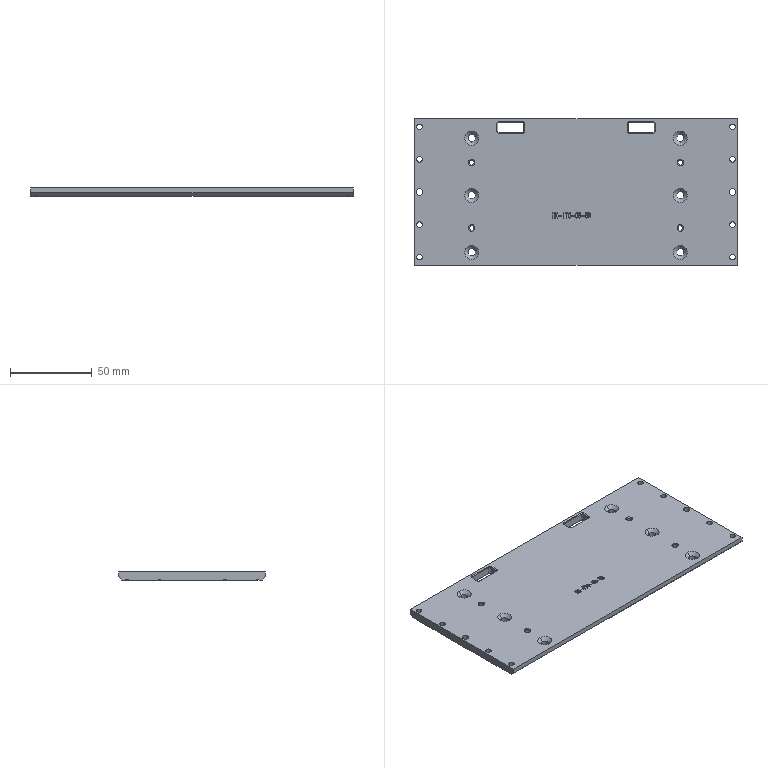NC program | NX | posted with a generic post | part box 198 x 90 x 5 mm
Lines 1352 to 3241 of 7160, first 1568 of 1886 lines:
(ZLEVEL_PROFILE_COPY_1_COPY_COPY_COPY , TOOL : D2)
N2654 T17 M6
N2656 G54
N2658 G17 G0 G90 X-34.395 Y37.9 S9500 M3
N2660 G43 Z30. H17
N2662 Z-0.2
N2664 G94 G1 X-34.222 Y37.6 F1000.
N2666 G3 X-34.048 Y37.5 R0.2
N2668 G1 X-32.9 F1100.
N2670 Y37.653
N2672 Y38.648
N2674 G3 X-33. Y38.822 R0.2
N2676 G1 X-33.3 Y38.995
N2678 G0 X-34.395 Y37.9 Z-0.4
N2680 G1 X-34.222 Y37.6 F1000.
N2682 G3 X-34.048 Y37.5 R0.2
N2684 G1 X-32.9 F1100.
N2686 Y37.653
N2688 Y38.648
N2690 G3 X-33. Y38.822 R0.2
N2692 G1 X-33.3 Y38.995
N2694 G0 X-34.395 Y37.9 Z-0.6
N2696 G1 X-34.222 Y37.6 F1000.
N2698 G3 X-34.048 Y37.5 R0.2
N2700 G1 X-32.9 F1100.
N2702 Y37.653
N2704 Y38.648
N2706 G3 X-33. Y38.822 R0.2
N2708 G1 X-33.3 Y38.995
N2710 G0 X-34.395 Y37.9 Z-0.8
N2712 G1 X-34.222 Y37.6 F1000.
N2714 G3 X-34.048 Y37.5 R0.2
N2716 G1 X-32.9 F1100.
N2718 Y37.653
N2720 Y38.648
N2722 G3 X-33. Y38.822 R0.2
N2724 G1 X-33.3 Y38.995
N2726 G0 X-34.395 Y37.9 Z-1.
N2728 G1 X-34.222 Y37.6 F1000.
N2730 G3 X-34.048 Y37.5 R0.2
N2732 G1 X-32.9 F1100.
N2734 Y37.653
N2736 Y38.648
N2738 G3 X-33. Y38.822 R0.2
N2740 G1 X-33.3 Y38.995
N2742 G0 X-34.395 Y37.9 Z-1.2
N2744 G1 X-34.222 Y37.6 F1000.
N2746 G3 X-34.048 Y37.5 R0.2
N2748 G1 X-32.9 F1100.
N2750 Y37.653
N2752 Y38.648
N2754 G3 X-33. Y38.822 R0.2
N2756 G1 X-33.3 Y38.995
N2758 G0 X-34.395 Y37.9 Z-1.4
N2760 G1 X-34.222 Y37.6 F1000.
N2762 G3 X-34.048 Y37.5 R0.2
N2764 G1 X-32.9 F1100.
N2766 Y37.653
N2768 Y38.648
N2770 G3 X-33. Y38.822 R0.2
N2772 G1 X-33.3 Y38.995
N2774 G0 X-34.395 Y37.9 Z-1.6
N2776 G1 X-34.222 Y37.6 F1000.
N2778 G3 X-34.048 Y37.5 R0.2
N2780 G1 X-32.9 F1100.
N2782 Y37.653
N2784 Y38.648
N2786 G3 X-33. Y38.822 R0.2
N2788 G1 X-33.3 Y38.995
N2790 G0 X-34.395 Y37.9 Z-1.8
N2792 G1 X-34.222 Y37.6 F1000.
N2794 G3 X-34.048 Y37.5 R0.2
N2796 G1 X-32.9 F1100.
N2798 Y37.653
N2800 Y38.648
N2802 G3 X-33. Y38.822 R0.2
N2804 G1 X-33.3 Y38.995
N2806 G0 X-34.395 Y37.9 Z-2.
N2808 G1 X-34.222 Y37.6 F1000.
N2810 G3 X-34.048 Y37.5 R0.2
N2812 G1 X-32.9 F1100.
N2814 Y37.653
N2816 Y38.648
N2818 G3 X-33. Y38.822 R0.2
N2820 G1 X-33.3 Y38.995
N2822 G0 X-34.395 Y37.9 Z-2.2
N2824 G1 X-34.222 Y37.6 F1000.
N2826 G3 X-34.048 Y37.5 R0.2
N2828 G1 X-32.9 F1100.
N2830 Y37.653
N2832 Y38.648
N2834 G3 X-33. Y38.822 R0.2
N2836 G1 X-33.3 Y38.995
N2838 G0 X-34.395 Y37.9 Z-2.4
N2840 G1 X-34.222 Y37.6 F1000.
N2842 G3 X-34.048 Y37.5 R0.2
N2844 G1 X-32.9 F1100.
N2846 Y37.653
N2848 Y38.648
N2850 G3 X-33. Y38.822 R0.2
N2852 G1 X-33.3 Y38.995
N2854 G0 X-34.395 Y37.9 Z-2.6
N2856 G1 X-34.222 Y37.6 F1000.
N2858 G3 X-34.048 Y37.5 R0.2
N2860 G1 X-32.9 F1100.
N2862 Y37.653
N2864 Y38.648
N2866 G3 X-33. Y38.822 R0.2
N2868 G1 X-33.3 Y38.995
N2870 G0 X-34.395 Y37.9 Z-2.8
N2872 G1 X-34.222 Y37.6 F1000.
N2874 G3 X-34.048 Y37.5 R0.2
N2876 G1 X-32.9 F1100.
N2878 Y37.653
N2880 Y38.648
N2882 G3 X-33. Y38.822 R0.2
N2884 G1 X-33.3 Y38.995
N2886 G0 X-34.395 Y37.9 Z-3.
N2888 G1 X-34.222 Y37.6 F1000.
N2890 G3 X-34.048 Y37.5 R0.2
N2892 G1 X-32.9 F1100.
N2894 Y37.653
N2896 Y38.648
N2898 G3 X-33. Y38.822 R0.2
N2900 G1 X-33.3 Y38.995
N2902 G0 X-34.395 Y37.9 Z-3.2
N2904 G1 X-34.222 Y37.6 F1000.
N2906 G3 X-34.048 Y37.5 R0.2
N2908 G1 X-32.9 F1100.
N2910 Y37.653
N2912 Y38.648
N2914 G3 X-33. Y38.822 R0.2
N2916 G1 X-33.3 Y38.995
N2918 G0 X-34.395 Y37.9 Z-3.4
N2920 G1 X-34.222 Y37.6 F1000.
N2922 G3 X-34.048 Y37.5 R0.2
N2924 G1 X-32.9 F1100.
N2926 Y37.653
N2928 Y38.648
N2930 G3 X-33. Y38.822 R0.2
N2932 G1 X-33.3 Y38.995
N2934 G0 X-34.395 Y37.9 Z-3.6
N2936 G1 X-34.222 Y37.6 F1000.
N2938 G3 X-34.048 Y37.5 R0.2
N2940 G1 X-32.9 F1100.
N2942 Y37.653
N2944 Y38.648
N2946 G3 X-33. Y38.822 R0.2
N2948 G1 X-33.3 Y38.995
N2950 G0 X-34.395 Y37.9 Z-3.8
N2952 G1 X-34.222 Y37.6 F1000.
N2954 G3 X-34.048 Y37.5 R0.2
N2956 G1 X-32.9 F1100.
N2958 Y37.653
N2960 Y38.648
N2962 G3 X-33. Y38.822 R0.2
N2964 G1 X-33.3 Y38.995
N2966 G0 X-34.395 Y37.9 Z-4.
N2968 G1 X-34.222 Y37.6 F1000.
N2970 G3 X-34.048 Y37.5 R0.2
N2972 G1 X-32.9 F1100.
N2974 Y37.653
N2976 Y38.648
N2978 G3 X-33. Y38.822 R0.2
N2980 G1 X-33.3 Y38.995
N2982 G0 X-34.395 Y37.9 Z-4.2
N2984 G1 X-34.222 Y37.6 F1000.
N2986 G3 X-34.048 Y37.5 R0.2
N2988 G1 X-32.9 F1100.
N2990 Y37.653
N2992 Y38.648
N2994 G3 X-33. Y38.822 R0.2
N2996 G1 X-33.3 Y38.995
N2998 G0 X-34.395 Y37.9 Z-4.4
N3000 G1 X-34.222 Y37.6 F1000.
N3002 G3 X-34.048 Y37.5 R0.2
N3004 G1 X-32.9 F1100.
N3006 Y37.653
N3008 Y38.648
N3010 G3 X-33. Y38.822 R0.2
N3012 G1 X-33.3 Y38.995
N3014 G0 X-34.395 Y37.9 Z-4.6
N3016 G1 X-34.222 Y37.6 F1000.
N3018 G3 X-34.048 Y37.5 R0.2
N3020 G1 X-32.9 F1100.
N3022 Y37.653
N3024 Y38.648
N3026 G3 X-33. Y38.822 R0.2
N3028 G1 X-33.3 Y38.995
N3030 G0 X-34.395 Y37.9 Z-4.8
N3032 G1 X-34.222 Y37.6 F1000.
N3034 G3 X-34.048 Y37.5 R0.2
N3036 G1 X-32.9 F1100.
N3038 Y37.653
N3040 Y38.648
N3042 G3 X-33. Y38.822 R0.2
N3044 G1 X-33.3 Y38.995
N3046 G0 X-34.395 Y37.9 Z-5.
N3048 G1 X-34.222 Y37.6 F1000.
N3050 G3 X-34.048 Y37.5 R0.2
N3052 G1 X-32.9 F1100.
N3054 Y37.653
N3056 Y38.648
N3058 G3 X-33. Y38.822 R0.2
N3060 G1 X-33.3 Y38.995
N3062 G0 Z30.
N3064 Y40.205
N3066 Z-0.2
N3068 G1 X-33. Y40.378 F1000.
N3070 G3 X-32.9 Y40.552 R0.2
N3072 G1 Y41.7 F1100.
N3074 X-33.046
N3076 X-34.048
N3078 G3 X-34.222 Y41.6 R0.2
N3080 G1 X-34.395 Y41.3
N3082 G0 X-33.3 Y40.205 Z-0.4
N3084 G1 X-33. Y40.378 F1000.
N3086 G3 X-32.9 Y40.552 R0.2
N3088 G1 Y41.7 F1100.
N3090 X-33.046
N3092 X-34.048
N3094 G3 X-34.222 Y41.6 R0.2
N3096 G1 X-34.395 Y41.3
N3098 G0 X-33.3 Y40.205 Z-0.6
N3100 G1 X-33. Y40.378 F1000.
N3102 G3 X-32.9 Y40.552 R0.2
N3104 G1 Y41.7 F1100.
N3106 X-33.046
N3108 X-34.048
N3110 G3 X-34.222 Y41.6 R0.2
N3112 G1 X-34.395 Y41.3
N3114 G0 X-33.3 Y40.205 Z-0.8
N3116 G1 X-33. Y40.378 F1000.
N3118 G3 X-32.9 Y40.552 R0.2
N3120 G1 Y41.7 F1100.
N3122 X-33.046
N3124 X-34.048
N3126 G3 X-34.222 Y41.6 R0.2
N3128 G1 X-34.395 Y41.3
N3130 G0 X-33.3 Y40.205 Z-1.
N3132 G1 X-33. Y40.378 F1000.
N3134 G3 X-32.9 Y40.552 R0.2
N3136 G1 Y41.7 F1100.
N3138 X-33.046
N3140 X-34.048
N3142 G3 X-34.222 Y41.6 R0.2
N3144 G1 X-34.395 Y41.3
N3146 G0 X-33.3 Y40.205 Z-1.2
N3148 G1 X-33. Y40.378 F1000.
N3150 G3 X-32.9 Y40.552 R0.2
N3152 G1 Y41.7 F1100.
N3154 X-33.046
N3156 X-34.048
N3158 G3 X-34.222 Y41.6 R0.2
N3160 G1 X-34.395 Y41.3
N3162 G0 X-33.3 Y40.205 Z-1.4
N3164 G1 X-33. Y40.378 F1000.
N3166 G3 X-32.9 Y40.552 R0.2
N3168 G1 Y41.7 F1100.
N3170 X-33.046
N3172 X-34.048
N3174 G3 X-34.222 Y41.6 R0.2
N3176 G1 X-34.395 Y41.3
N3178 G0 X-33.3 Y40.205 Z-1.6
N3180 G1 X-33. Y40.378 F1000.
N3182 G3 X-32.9 Y40.552 R0.2
N3184 G1 Y41.7 F1100.
N3186 X-33.046
N3188 X-34.048
N3190 G3 X-34.222 Y41.6 R0.2
N3192 G1 X-34.395 Y41.3
N3194 G0 X-33.3 Y40.205 Z-1.8
N3196 G1 X-33. Y40.378 F1000.
N3198 G3 X-32.9 Y40.552 R0.2
N3200 G1 Y41.7 F1100.
N3202 X-33.046
N3204 X-34.048
N3206 G3 X-34.222 Y41.6 R0.2
N3208 G1 X-34.395 Y41.3
N3210 G0 X-33.3 Y40.205 Z-2.
N3212 G1 X-33. Y40.378 F1000.
N3214 G3 X-32.9 Y40.552 R0.2
N3216 G1 Y41.7 F1100.
N3218 X-33.046
N3220 X-34.048
N3222 G3 X-34.222 Y41.6 R0.2
N3224 G1 X-34.395 Y41.3
N3226 G0 X-33.3 Y40.205 Z-2.2
N3228 G1 X-33. Y40.378 F1000.
N3230 G3 X-32.9 Y40.552 R0.2
N3232 G1 Y41.7 F1100.
N3234 X-33.046
N3236 X-34.048
N3238 G3 X-34.222 Y41.6 R0.2
N3240 G1 X-34.395 Y41.3
N3242 G0 X-33.3 Y40.205 Z-2.4
N3244 G1 X-33. Y40.378 F1000.
N3246 G3 X-32.9 Y40.552 R0.2
N3248 G1 Y41.7 F1100.
N3250 X-33.046
N3252 X-34.048
N3254 G3 X-34.222 Y41.6 R0.2
N3256 G1 X-34.395 Y41.3
N3258 G0 X-33.3 Y40.205 Z-2.6
N3260 G1 X-33. Y40.378 F1000.
N3262 G3 X-32.9 Y40.552 R0.2
N3264 G1 Y41.7 F1100.
N3266 X-33.046
N3268 X-34.048
N3270 G3 X-34.222 Y41.6 R0.2
N3272 G1 X-34.395 Y41.3
N3274 G0 X-33.3 Y40.205 Z-2.8
N3276 G1 X-33. Y40.378 F1000.
N3278 G3 X-32.9 Y40.552 R0.2
N3280 G1 Y41.7 F1100.
N3282 X-33.046
N3284 X-34.048
N3286 G3 X-34.222 Y41.6 R0.2
N3288 G1 X-34.395 Y41.3
N3290 G0 X-33.3 Y40.205 Z-3.
N3292 G1 X-33. Y40.378 F1000.
N3294 G3 X-32.9 Y40.552 R0.2
N3296 G1 Y41.7 F1100.
N3298 X-33.046
N3300 X-34.048
N3302 G3 X-34.222 Y41.6 R0.2
N3304 G1 X-34.395 Y41.3
N3306 G0 X-33.3 Y40.205 Z-3.2
N3308 G1 X-33. Y40.378 F1000.
N3310 G3 X-32.9 Y40.552 R0.2
N3312 G1 Y41.7 F1100.
N3314 X-33.046
N3316 X-34.048
N3318 G3 X-34.222 Y41.6 R0.2
N3320 G1 X-34.395 Y41.3
N3322 G0 X-33.3 Y40.205 Z-3.4
N3324 G1 X-33. Y40.378 F1000.
N3326 G3 X-32.9 Y40.552 R0.2
N3328 G1 Y41.7 F1100.
N3330 X-33.046
N3332 X-34.048
N3334 G3 X-34.222 Y41.6 R0.2
N3336 G1 X-34.395 Y41.3
N3338 G0 X-33.3 Y40.205 Z-3.6
N3340 G1 X-33. Y40.378 F1000.
N3342 G3 X-32.9 Y40.552 R0.2
N3344 G1 Y41.7 F1100.
N3346 X-33.046
N3348 X-34.048
N3350 G3 X-34.222 Y41.6 R0.2
N3352 G1 X-34.395 Y41.3
N3354 G0 X-33.3 Y40.205 Z-3.8
N3356 G1 X-33. Y40.378 F1000.
N3358 G3 X-32.9 Y40.552 R0.2
N3360 G1 Y41.7 F1100.
N3362 X-33.046
N3364 X-34.048
N3366 G3 X-34.222 Y41.6 R0.2
N3368 G1 X-34.395 Y41.3
N3370 G0 X-33.3 Y40.205 Z-4.
N3372 G1 X-33. Y40.378 F1000.
N3374 G3 X-32.9 Y40.552 R0.2
N3376 G1 Y41.7 F1100.
N3378 X-33.003
N3380 X-34.048
N3382 G3 X-34.222 Y41.6 R0.2
N3384 G1 X-34.395 Y41.3
N3386 G0 X-33.3 Y40.205 Z-4.2
N3388 G1 X-33. Y40.378 F1000.
N3390 G3 X-32.9 Y40.552 R0.2
N3392 G1 Y41.7 F1100.
N3394 X-33.003
N3396 X-34.048
N3398 G3 X-34.222 Y41.6 R0.2
N3400 G1 X-34.395 Y41.3
N3402 G0 X-33.3 Y40.205 Z-4.4
N3404 G1 X-33. Y40.378 F1000.
N3406 G3 X-32.9 Y40.552 R0.2
N3408 G1 Y41.7 F1100.
N3410 X-33.003
N3412 X-34.048
N3414 G3 X-34.222 Y41.6 R0.2
N3416 G1 X-34.395 Y41.3
N3418 G0 X-33.3 Y40.206 Z-4.6
N3420 G1 X-33. Y40.379 F1000.
N3422 G3 X-32.9 Y40.552 R0.2
N3424 G1 Y41.7 F1100.
N3426 X-34.048
N3428 G3 X-34.221 Y41.6 R0.2
N3430 G1 X-34.394 Y41.3
N3432 G0 X-33.3 Y40.206 Z-4.8
N3434 G1 X-33. Y40.379 F1000.
N3436 G3 X-32.9 Y40.552 R0.2
N3438 G1 Y41.7 F1100.
N3440 X-34.048
N3442 G3 X-34.221 Y41.6 R0.2
N3444 G1 X-34.394 Y41.3
N3446 G0 X-33.3 Y40.206 Z-5.
N3448 G1 X-33. Y40.379 F1000.
N3450 G3 X-32.9 Y40.552 R0.2
N3452 G1 Y41.7 F1100.
N3454 X-34.048
N3456 G3 X-34.221 Y41.6 R0.2
N3458 G1 X-34.394 Y41.3
N3460 G0 Z30.
N3462 X-45.605
N3464 Z-0.2
N3466 G1 X-45.778 Y41.6 F1000.
N3468 G3 X-45.952 Y41.7 R0.2
N3470 G1 X-46.954 F1100.
N3472 X-47.1
N3474 Y40.552
N3476 G3 X-47. Y40.378 R0.2
N3478 G1 X-46.7 Y40.205
N3480 G0 X-45.605 Y41.3 Z-0.4
N3482 G1 X-45.778 Y41.6 F1000.
N3484 G3 X-45.952 Y41.7 R0.2
N3486 G1 X-46.954 F1100.
N3488 X-47.1
N3490 Y40.552
N3492 G3 X-47. Y40.378 R0.2
N3494 G1 X-46.7 Y40.205
N3496 G0 X-45.605 Y41.3 Z-0.6
N3498 G1 X-45.778 Y41.6 F1000.
N3500 G3 X-45.952 Y41.7 R0.2
N3502 G1 X-46.954 F1100.
N3504 X-47.1
N3506 Y40.552
N3508 G3 X-47. Y40.378 R0.2
N3510 G1 X-46.7 Y40.205
N3512 G0 X-45.605 Y41.3 Z-0.8
N3514 G1 X-45.778 Y41.6 F1000.
N3516 G3 X-45.952 Y41.7 R0.2
N3518 G1 X-46.954 F1100.
N3520 X-47.1
N3522 Y40.552
N3524 G3 X-47. Y40.378 R0.2
N3526 G1 X-46.7 Y40.205
N3528 G0 X-45.605 Y41.3 Z-1.
N3530 G1 X-45.778 Y41.6 F1000.
N3532 G3 X-45.952 Y41.7 R0.2
N3534 G1 X-46.954 F1100.
N3536 X-47.1
N3538 Y40.552
N3540 G3 X-47. Y40.378 R0.2
N3542 G1 X-46.7 Y40.205
N3544 G0 X-45.605 Y41.3 Z-1.2
N3546 G1 X-45.778 Y41.6 F1000.
N3548 G3 X-45.952 Y41.7 R0.2
N3550 G1 X-46.954 F1100.
N3552 X-47.1
N3554 Y40.552
N3556 G3 X-47. Y40.378 R0.2
N3558 G1 X-46.7 Y40.205
N3560 G0 X-45.605 Y41.3 Z-1.4
N3562 G1 X-45.778 Y41.6 F1000.
N3564 G3 X-45.952 Y41.7 R0.2
N3566 G1 X-46.954 F1100.
N3568 X-47.1
N3570 Y40.552
N3572 G3 X-47. Y40.378 R0.2
N3574 G1 X-46.7 Y40.205
N3576 G0 X-45.605 Y41.3 Z-1.6
N3578 G1 X-45.778 Y41.6 F1000.
N3580 G3 X-45.952 Y41.7 R0.2
N3582 G1 X-46.954 F1100.
N3584 X-47.1
N3586 Y40.552
N3588 G3 X-47. Y40.378 R0.2
N3590 G1 X-46.7 Y40.205
N3592 G0 X-45.605 Y41.3 Z-1.8
N3594 G1 X-45.778 Y41.6 F1000.
N3596 G3 X-45.952 Y41.7 R0.2
N3598 G1 X-46.954 F1100.
N3600 X-47.1
N3602 Y40.552
N3604 G3 X-47. Y40.378 R0.2
N3606 G1 X-46.7 Y40.205
N3608 G0 X-45.605 Y41.3 Z-2.
N3610 G1 X-45.778 Y41.6 F1000.
N3612 G3 X-45.952 Y41.7 R0.2
N3614 G1 X-46.954 F1100.
N3616 X-47.1
N3618 Y40.552
N3620 G3 X-47. Y40.378 R0.2
N3622 G1 X-46.7 Y40.205
N3624 G0 X-45.605 Y41.3 Z-2.2
N3626 G1 X-45.778 Y41.6 F1000.
N3628 G3 X-45.952 Y41.7 R0.2
N3630 G1 X-46.954 F1100.
N3632 X-47.1
N3634 Y40.552
N3636 G3 X-47. Y40.378 R0.2
N3638 G1 X-46.7 Y40.205
N3640 G0 X-45.605 Y41.3 Z-2.4
N3642 G1 X-45.778 Y41.6 F1000.
N3644 G3 X-45.952 Y41.7 R0.2
N3646 G1 X-46.954 F1100.
N3648 X-47.1
N3650 Y40.552
N3652 G3 X-47. Y40.378 R0.2
N3654 G1 X-46.7 Y40.205
N3656 G0 X-45.605 Y41.3 Z-2.6
N3658 G1 X-45.778 Y41.6 F1000.
N3660 G3 X-45.952 Y41.7 R0.2
N3662 G1 X-46.954 F1100.
N3664 X-47.1
N3666 Y40.552
N3668 G3 X-47. Y40.378 R0.2
N3670 G1 X-46.7 Y40.205
N3672 G0 X-45.605 Y41.3 Z-2.8
N3674 G1 X-45.778 Y41.6 F1000.
N3676 G3 X-45.952 Y41.7 R0.2
N3678 G1 X-46.954 F1100.
N3680 X-47.1
N3682 Y40.552
N3684 G3 X-47. Y40.378 R0.2
N3686 G1 X-46.7 Y40.205
N3688 G0 X-45.605 Y41.3 Z-3.
N3690 G1 X-45.778 Y41.6 F1000.
N3692 G3 X-45.952 Y41.7 R0.2
N3694 G1 X-46.954 F1100.
N3696 X-47.1
N3698 Y40.552
N3700 G3 X-47. Y40.378 R0.2
N3702 G1 X-46.7 Y40.205
N3704 G0 X-45.605 Y41.3 Z-3.2
N3706 G1 X-45.778 Y41.6 F1000.
N3708 G3 X-45.952 Y41.7 R0.2
N3710 G1 X-46.954 F1100.
N3712 X-47.1
N3714 Y40.552
N3716 G3 X-47. Y40.378 R0.2
N3718 G1 X-46.7 Y40.205
N3720 G0 X-45.605 Y41.3 Z-3.4
N3722 G1 X-45.778 Y41.6 F1000.
N3724 G3 X-45.952 Y41.7 R0.2
N3726 G1 X-46.954 F1100.
N3728 X-47.1
N3730 Y40.552
N3732 G3 X-47. Y40.378 R0.2
N3734 G1 X-46.7 Y40.205
N3736 G0 X-45.605 Y41.3 Z-3.6
N3738 G1 X-45.778 Y41.6 F1000.
N3740 G3 X-45.952 Y41.7 R0.2
N3742 G1 X-46.954 F1100.
N3744 X-47.1
N3746 Y40.552
N3748 G3 X-47. Y40.378 R0.2
N3750 G1 X-46.7 Y40.205
N3752 G0 X-45.605 Y41.3 Z-3.8
N3754 G1 X-45.778 Y41.6 F1000.
N3756 G3 X-45.952 Y41.7 R0.2
N3758 G1 X-46.954 F1100.
N3760 X-47.1
N3762 Y40.552
N3764 G3 X-47. Y40.378 R0.2
N3766 G1 X-46.7 Y40.205
N3768 G0 X-45.605 Y41.3 Z-4.
N3770 G1 X-45.778 Y41.6 F1000.
N3772 G3 X-45.952 Y41.7 R0.2
N3774 G1 X-46.997 F1100.
N3776 X-47.1
N3778 Y40.552
N3780 G3 X-47. Y40.378 R0.2
N3782 G1 X-46.7 Y40.205
N3784 G0 X-45.605 Y41.3 Z-4.2
N3786 G1 X-45.778 Y41.6 F1000.
N3788 G3 X-45.952 Y41.7 R0.2
N3790 G1 X-46.997 F1100.
N3792 X-47.1
N3794 Y40.552
N3796 G3 X-47. Y40.378 R0.2
N3798 G1 X-46.7 Y40.205
N3800 G0 X-45.605 Y41.3 Z-4.4
N3802 G1 X-45.778 Y41.6 F1000.
N3804 G3 X-45.952 Y41.7 R0.2
N3806 G1 X-46.997 F1100.
N3808 X-47.1
N3810 Y40.552
N3812 G3 X-47. Y40.378 R0.2
N3814 G1 X-46.7 Y40.205
N3816 G0 X-45.605 Y41.3 Z-4.6
N3818 G1 X-45.778 Y41.6 F1000.
N3820 G3 X-45.952 Y41.7 R0.2
N3822 G1 X-47.1 F1100.
N3824 Y40.552
N3826 G3 X-47. Y40.378 R0.2
N3828 G1 X-46.7 Y40.205
N3830 G0 X-45.605 Y41.3 Z-4.8
N3832 G1 X-45.778 Y41.6 F1000.
N3834 G3 X-45.952 Y41.7 R0.2
N3836 G1 X-47.1 F1100.
N3838 Y40.552
N3840 G3 X-47. Y40.378 R0.2
N3842 G1 X-46.7 Y40.205
N3844 G0 X-45.605 Y41.3 Z-5.
N3846 G1 X-45.778 Y41.6 F1000.
N3848 G3 X-45.952 Y41.7 R0.2
N3850 G1 X-47.1 F1100.
N3852 Y40.552
N3854 G3 X-47. Y40.378 R0.2
N3856 G1 X-46.7 Y40.205
N3858 G0 Z30.
N3860 Y38.995
N3862 Z-0.2
N3864 G1 X-47. Y38.822 F1000.
N3866 G3 X-47.1 Y38.648 R0.2
N3868 G1 Y37.653 F1100.
N3870 Y37.5
N3872 X-45.952
N3874 G3 X-45.778 Y37.6 R0.2
N3876 G1 X-45.605 Y37.9
N3878 G0 X-46.7 Y38.995 Z-0.4
N3880 G1 X-47. Y38.822 F1000.
N3882 G3 X-47.1 Y38.648 R0.2
N3884 G1 Y37.653 F1100.
N3886 Y37.5
N3888 X-45.952
N3890 G3 X-45.778 Y37.6 R0.2
N3892 G1 X-45.605 Y37.9
N3894 G0 X-46.7 Y38.995 Z-0.6
N3896 G1 X-47. Y38.822 F1000.
N3898 G3 X-47.1 Y38.648 R0.2
N3900 G1 Y37.653 F1100.
N3902 Y37.5
N3904 X-45.952
N3906 G3 X-45.778 Y37.6 R0.2
N3908 G1 X-45.605 Y37.9
N3910 G0 X-46.7 Y38.995 Z-0.8
N3912 G1 X-47. Y38.822 F1000.
N3914 G3 X-47.1 Y38.648 R0.2
N3916 G1 Y37.653 F1100.
N3918 Y37.5
N3920 X-45.952
N3922 G3 X-45.778 Y37.6 R0.2
N3924 G1 X-45.605 Y37.9
N3926 G0 X-46.7 Y38.995 Z-1.
N3928 G1 X-47. Y38.822 F1000.
N3930 G3 X-47.1 Y38.648 R0.2
N3932 G1 Y37.653 F1100.
N3934 Y37.5
N3936 X-45.952
N3938 G3 X-45.778 Y37.6 R0.2
N3940 G1 X-45.605 Y37.9
N3942 G0 X-46.7 Y38.995 Z-1.2
N3944 G1 X-47. Y38.822 F1000.
N3946 G3 X-47.1 Y38.648 R0.2
N3948 G1 Y37.653 F1100.
N3950 Y37.5
N3952 X-45.952
N3954 G3 X-45.778 Y37.6 R0.2
N3956 G1 X-45.605 Y37.9
N3958 G0 X-46.7 Y38.995 Z-1.4
N3960 G1 X-47. Y38.822 F1000.
N3962 G3 X-47.1 Y38.648 R0.2
N3964 G1 Y37.653 F1100.
N3966 Y37.5
N3968 X-45.952
N3970 G3 X-45.778 Y37.6 R0.2
N3972 G1 X-45.605 Y37.9
N3974 G0 X-46.7 Y38.995 Z-1.6
N3976 G1 X-47. Y38.822 F1000.
N3978 G3 X-47.1 Y38.648 R0.2
N3980 G1 Y37.653 F1100.
N3982 Y37.5
N3984 X-45.952
N3986 G3 X-45.778 Y37.6 R0.2
N3988 G1 X-45.605 Y37.9
N3990 G0 X-46.7 Y38.995 Z-1.8
N3992 G1 X-47. Y38.822 F1000.
N3994 G3 X-47.1 Y38.648 R0.2
N3996 G1 Y37.653 F1100.
N3998 Y37.5
N4000 X-45.952
N4002 G3 X-45.778 Y37.6 R0.2
N4004 G1 X-45.605 Y37.9
N4006 G0 X-46.7 Y38.995 Z-2.
N4008 G1 X-47. Y38.822 F1000.
N4010 G3 X-47.1 Y38.648 R0.2
N4012 G1 Y37.653 F1100.
N4014 Y37.5
N4016 X-45.952
N4018 G3 X-45.778 Y37.6 R0.2
N4020 G1 X-45.605 Y37.9
N4022 G0 X-46.7 Y38.995 Z-2.2
N4024 G1 X-47. Y38.822 F1000.
N4026 G3 X-47.1 Y38.648 R0.2
N4028 G1 Y37.653 F1100.
N4030 Y37.5
N4032 X-45.952
N4034 G3 X-45.778 Y37.6 R0.2
N4036 G1 X-45.605 Y37.9
N4038 G0 X-46.7 Y38.995 Z-2.4
N4040 G1 X-47. Y38.822 F1000.
N4042 G3 X-47.1 Y38.648 R0.2
N4044 G1 Y37.653 F1100.
N4046 Y37.5
N4048 X-45.952
N4050 G3 X-45.778 Y37.6 R0.2
N4052 G1 X-45.605 Y37.9
N4054 G0 X-46.7 Y38.995 Z-2.6
N4056 G1 X-47. Y38.822 F1000.
N4058 G3 X-47.1 Y38.648 R0.2
N4060 G1 Y37.653 F1100.
N4062 Y37.5
N4064 X-45.952
N4066 G3 X-45.778 Y37.6 R0.2
N4068 G1 X-45.605 Y37.9
N4070 G0 X-46.7 Y38.995 Z-2.8
N4072 G1 X-47. Y38.822 F1000.
N4074 G3 X-47.1 Y38.648 R0.2
N4076 G1 Y37.653 F1100.
N4078 Y37.5
N4080 X-45.952
N4082 G3 X-45.778 Y37.6 R0.2
N4084 G1 X-45.605 Y37.9
N4086 G0 X-46.7 Y38.995 Z-3.
N4088 G1 X-47. Y38.822 F1000.
N4090 G3 X-47.1 Y38.648 R0.2
N4092 G1 Y37.653 F1100.
N4094 Y37.5
N4096 X-45.952
N4098 G3 X-45.778 Y37.6 R0.2
N4100 G1 X-45.605 Y37.9
N4102 G0 X-46.7 Y38.995 Z-3.2
N4104 G1 X-47. Y38.822 F1000.
N4106 G3 X-47.1 Y38.648 R0.2
N4108 G1 Y37.653 F1100.
N4110 Y37.5
N4112 X-45.952
N4114 G3 X-45.778 Y37.6 R0.2
N4116 G1 X-45.605 Y37.9
N4118 G0 X-46.7 Y38.995 Z-3.4
N4120 G1 X-47. Y38.822 F1000.
N4122 G3 X-47.1 Y38.648 R0.2
N4124 G1 Y37.653 F1100.
N4126 Y37.5
N4128 X-45.952
N4130 G3 X-45.778 Y37.6 R0.2
N4132 G1 X-45.605 Y37.9
N4134 G0 X-46.7 Y38.995 Z-3.6
N4136 G1 X-47. Y38.822 F1000.
N4138 G3 X-47.1 Y38.648 R0.2
N4140 G1 Y37.653 F1100.
N4142 Y37.5
N4144 X-45.952
N4146 G3 X-45.778 Y37.6 R0.2
N4148 G1 X-45.605 Y37.9
N4150 G0 X-46.7 Y38.995 Z-3.8
N4152 G1 X-47. Y38.822 F1000.
N4154 G3 X-47.1 Y38.648 R0.2
N4156 G1 Y37.653 F1100.
N4158 Y37.5
N4160 X-45.952
N4162 G3 X-45.778 Y37.6 R0.2
N4164 G1 X-45.605 Y37.9
N4166 G0 X-46.7 Y38.995 Z-4.
N4168 G1 X-47. Y38.822 F1000.
N4170 G3 X-47.1 Y38.648 R0.2
N4172 G1 Y37.653 F1100.
N4174 Y37.5
N4176 X-45.952
N4178 G3 X-45.778 Y37.6 R0.2
N4180 G1 X-45.605 Y37.9
N4182 G0 X-46.7 Y38.995 Z-4.2
N4184 G1 X-47. Y38.822 F1000.
N4186 G3 X-47.1 Y38.648 R0.2
N4188 G1 Y37.653 F1100.
N4190 Y37.5
N4192 X-45.952
N4194 G3 X-45.778 Y37.6 R0.2
N4196 G1 X-45.605 Y37.9
N4198 G0 X-46.7 Y38.995 Z-4.4
N4200 G1 X-47. Y38.822 F1000.
N4202 G3 X-47.1 Y38.648 R0.2
N4204 G1 Y37.653 F1100.
N4206 Y37.5
N4208 X-45.952
N4210 G3 X-45.778 Y37.6 R0.2
N4212 G1 X-45.605 Y37.9
N4214 G0 X-46.7 Y38.994 Z-4.6
N4216 G1 X-47. Y38.821 F1000.
N4218 G3 X-47.1 Y38.647 R0.2
N4220 G1 Y37.653 F1100.
N4222 Y37.5
N4224 X-45.953
N4226 G3 X-45.779 Y37.6 R0.2
N4228 G1 X-45.606 Y37.9
N4230 G0 X-46.7 Y38.994 Z-4.8
N4232 G1 X-47. Y38.821 F1000.
N4234 G3 X-47.1 Y38.647 R0.2
N4236 G1 Y37.653 F1100.
N4238 Y37.5
N4240 X-45.953
N4242 G3 X-45.779 Y37.6 R0.2
N4244 G1 X-45.606 Y37.9
N4246 G0 X-46.7 Y38.994 Z-5.
N4248 G1 X-47. Y38.821 F1000.
N4250 G3 X-47.1 Y38.647 R0.2
N4252 G1 Y37.653 F1100.
N4254 Y37.5
N4256 X-45.953
N4258 G3 X-45.779 Y37.6 R0.2
N4260 G1 X-45.606 Y37.9
N4262 G0 Z30.
N4264 X45.605
N4266 Z-0.2
N4268 G1 X45.778 Y37.6 F1000.
N4270 G3 X45.952 Y37.5 R0.2
N4272 G1 X47.1 F1100.
N4274 Y37.653
N4276 Y38.648
N4278 G3 X47. Y38.822 R0.2
N4280 G1 X46.7 Y38.995
N4282 G0 X45.605 Y37.9 Z-0.4
N4284 G1 X45.778 Y37.6 F1000.
N4286 G3 X45.952 Y37.5 R0.2
N4288 G1 X47.1 F1100.
N4290 Y37.653
N4292 Y38.648
N4294 G3 X47. Y38.822 R0.2
N4296 G1 X46.7 Y38.995
N4298 G0 X45.605 Y37.9 Z-0.6
N4300 G1 X45.778 Y37.6 F1000.
N4302 G3 X45.952 Y37.5 R0.2
N4304 G1 X47.1 F1100.
N4306 Y37.653
N4308 Y38.648
N4310 G3 X47. Y38.822 R0.2
N4312 G1 X46.7 Y38.995
N4314 G0 X45.605 Y37.9 Z-0.8
N4316 G1 X45.778 Y37.6 F1000.
N4318 G3 X45.952 Y37.5 R0.2
N4320 G1 X47.1 F1100.
N4322 Y37.653
N4324 Y38.648
N4326 G3 X47. Y38.822 R0.2
N4328 G1 X46.7 Y38.995
N4330 G0 X45.605 Y37.9 Z-1.
N4332 G1 X45.778 Y37.6 F1000.
N4334 G3 X45.952 Y37.5 R0.2
N4336 G1 X47.1 F1100.
N4338 Y37.653
N4340 Y38.648
N4342 G3 X47. Y38.822 R0.2
N4344 G1 X46.7 Y38.995
N4346 G0 X45.605 Y37.9 Z-1.2
N4348 G1 X45.778 Y37.6 F1000.
N4350 G3 X45.952 Y37.5 R0.2
N4352 G1 X47.1 F1100.
N4354 Y37.653
N4356 Y38.648
N4358 G3 X47. Y38.822 R0.2
N4360 G1 X46.7 Y38.995
N4362 G0 X45.605 Y37.9 Z-1.4
N4364 G1 X45.778 Y37.6 F1000.
N4366 G3 X45.952 Y37.5 R0.2
N4368 G1 X47.1 F1100.
N4370 Y37.653
N4372 Y38.648
N4374 G3 X47. Y38.822 R0.2
N4376 G1 X46.7 Y38.995
N4378 G0 X45.605 Y37.9 Z-1.6
N4380 G1 X45.778 Y37.6 F1000.
N4382 G3 X45.952 Y37.5 R0.2
N4384 G1 X47.1 F1100.
N4386 Y37.653
N4388 Y38.648
N4390 G3 X47. Y38.822 R0.2
N4392 G1 X46.7 Y38.995
N4394 G0 X45.605 Y37.9 Z-1.8
N4396 G1 X45.778 Y37.6 F1000.
N4398 G3 X45.952 Y37.5 R0.2
N4400 G1 X47.1 F1100.
N4402 Y37.653
N4404 Y38.648
N4406 G3 X47. Y38.822 R0.2
N4408 G1 X46.7 Y38.995
N4410 G0 X45.605 Y37.9 Z-2.
N4412 G1 X45.778 Y37.6 F1000.
N4414 G3 X45.952 Y37.5 R0.2
N4416 G1 X47.1 F1100.
N4418 Y37.653
N4420 Y38.648
N4422 G3 X47. Y38.822 R0.2
N4424 G1 X46.7 Y38.995
N4426 G0 X45.605 Y37.9 Z-2.2
N4428 G1 X45.778 Y37.6 F1000.
N4430 G3 X45.952 Y37.5 R0.2
N4432 G1 X47.1 F1100.
N4434 Y37.653
N4436 Y38.648
N4438 G3 X47. Y38.822 R0.2
N4440 G1 X46.7 Y38.995
N4442 G0 X45.605 Y37.9 Z-2.4
N4444 G1 X45.778 Y37.6 F1000.
N4446 G3 X45.952 Y37.5 R0.2
N4448 G1 X47.1 F1100.
N4450 Y37.653
N4452 Y38.648
N4454 G3 X47. Y38.822 R0.2
N4456 G1 X46.7 Y38.995
N4458 G0 X45.605 Y37.9 Z-2.6
N4460 G1 X45.778 Y37.6 F1000.
N4462 G3 X45.952 Y37.5 R0.2
N4464 G1 X47.1 F1100.
N4466 Y37.653
N4468 Y38.648
N4470 G3 X47. Y38.822 R0.2
N4472 G1 X46.7 Y38.995
N4474 G0 X45.605 Y37.9 Z-2.8
N4476 G1 X45.778 Y37.6 F1000.
N4478 G3 X45.952 Y37.5 R0.2
N4480 G1 X47.1 F1100.
N4482 Y37.653
N4484 Y38.648
N4486 G3 X47. Y38.822 R0.2
N4488 G1 X46.7 Y38.995
N4490 G0 X45.605 Y37.9 Z-3.
N4492 G1 X45.778 Y37.6 F1000.
N4494 G3 X45.952 Y37.5 R0.2
N4496 G1 X47.1 F1100.
N4498 Y37.653
N4500 Y38.648
N4502 G3 X47. Y38.822 R0.2
N4504 G1 X46.7 Y38.995
N4506 G0 X45.605 Y37.9 Z-3.2
N4508 G1 X45.778 Y37.6 F1000.
N4510 G3 X45.952 Y37.5 R0.2
N4512 G1 X47.1 F1100.
N4514 Y37.653
N4516 Y38.648
N4518 G3 X47. Y38.822 R0.2
N4520 G1 X46.7 Y38.995
N4522 G0 X45.605 Y37.9 Z-3.4
N4524 G1 X45.778 Y37.6 F1000.
N4526 G3 X45.952 Y37.5 R0.2
N4528 G1 X47.1 F1100.
N4530 Y37.653
N4532 Y38.648
N4534 G3 X47. Y38.822 R0.2
N4536 G1 X46.7 Y38.995
N4538 G0 X45.605 Y37.9 Z-3.6
N4540 G1 X45.778 Y37.6 F1000.
N4542 G3 X45.952 Y37.5 R0.2
N4544 G1 X47.1 F1100.
N4546 Y37.653
N4548 Y38.648
N4550 G3 X47. Y38.822 R0.2
N4552 G1 X46.7 Y38.995
N4554 G0 X45.605 Y37.9 Z-3.8
N4556 G1 X45.778 Y37.6 F1000.
N4558 G3 X45.952 Y37.5 R0.2
N4560 G1 X47.1 F1100.
N4562 Y37.653
N4564 Y38.648
N4566 G3 X47. Y38.822 R0.2
N4568 G1 X46.7 Y38.995
N4570 G0 X45.605 Y37.9 Z-4.
N4572 G1 X45.778 Y37.6 F1000.
N4574 G3 X45.952 Y37.5 R0.2
N4576 G1 X47.1 F1100.
N4578 Y37.653
N4580 Y38.648
N4582 G3 X47. Y38.822 R0.2
N4584 G1 X46.7 Y38.995
N4586 G0 X45.605 Y37.9 Z-4.2
N4588 G1 X45.778 Y37.6 F1000.
N4590 G3 X45.952 Y37.5 R0.2
N4592 G1 X47.1 F1100.
N4594 Y37.653
N4596 Y38.648
N4598 G3 X47. Y38.822 R0.2
N4600 G1 X46.7 Y38.995
N4602 G0 X45.605 Y37.9 Z-4.4
N4604 G1 X45.778 Y37.6 F1000.
N4606 G3 X45.952 Y37.5 R0.2
N4608 G1 X47.1 F1100.
N4610 Y37.653
N4612 Y38.648
N4614 G3 X47. Y38.822 R0.2
N4616 G1 X46.7 Y38.995
N4618 G0 X45.606 Y37.9 Z-4.6
N4620 G1 X45.779 Y37.6 F1000.
N4622 G3 X45.953 Y37.5 R0.2
N4624 G1 X47.1 F1100.
N4626 Y37.653
N4628 Y38.647
N4630 G3 X47. Y38.821 R0.2
N4632 G1 X46.7 Y38.994
N4634 G0 X45.606 Y37.9 Z-4.8
N4636 G1 X45.779 Y37.6 F1000.
N4638 G3 X45.953 Y37.5 R0.2
N4640 G1 X47.1 F1100.
N4642 Y37.653
N4644 Y38.647
N4646 G3 X47. Y38.821 R0.2
N4648 G1 X46.7 Y38.994
N4650 G0 X45.606 Y37.9 Z-5.
N4652 G1 X45.779 Y37.6 F1000.
N4654 G3 X45.953 Y37.5 R0.2
N4656 G1 X47.1 F1100.
N4658 Y37.653
N4660 Y38.647
N4662 G3 X47. Y38.821 R0.2
N4664 G1 X46.7 Y38.994
N4666 G0 Z30.
N4668 Y40.205
N4670 Z-0.2
N4672 G1 X47. Y40.378 F1000.
N4674 G3 X47.1 Y40.552 R0.2
N4676 G1 Y41.7 F1100.
N4678 X46.954
N4680 X45.952
N4682 G3 X45.778 Y41.6 R0.2
N4684 G1 X45.605 Y41.3
N4686 G0 X46.7 Y40.205 Z-0.4
N4688 G1 X47. Y40.378 F1000.
N4690 G3 X47.1 Y40.552 R0.2
N4692 G1 Y41.7 F1100.
N4694 X46.954
N4696 X45.952
N4698 G3 X45.778 Y41.6 R0.2
N4700 G1 X45.605 Y41.3
N4702 G0 X46.7 Y40.205 Z-0.6
N4704 G1 X47. Y40.378 F1000.
N4706 G3 X47.1 Y40.552 R0.2
N4708 G1 Y41.7 F1100.
N4710 X46.954
N4712 X45.952
N4714 G3 X45.778 Y41.6 R0.2
N4716 G1 X45.605 Y41.3
N4718 G0 X46.7 Y40.205 Z-0.8
N4720 G1 X47. Y40.378 F1000.
N4722 G3 X47.1 Y40.552 R0.2
N4724 G1 Y41.7 F1100.
N4726 X46.954
N4728 X45.952
N4730 G3 X45.778 Y41.6 R0.2
N4732 G1 X45.605 Y41.3
N4734 G0 X46.7 Y40.205 Z-1.
N4736 G1 X47. Y40.378 F1000.
N4738 G3 X47.1 Y40.552 R0.2
N4740 G1 Y41.7 F1100.
N4742 X46.954
N4744 X45.952
N4746 G3 X45.778 Y41.6 R0.2
N4748 G1 X45.605 Y41.3
N4750 G0 X46.7 Y40.205 Z-1.2
N4752 G1 X47. Y40.378 F1000.
N4754 G3 X47.1 Y40.552 R0.2
N4756 G1 Y41.7 F1100.
N4758 X46.954
N4760 X45.952
N4762 G3 X45.778 Y41.6 R0.2
N4764 G1 X45.605 Y41.3
N4766 G0 X46.7 Y40.205 Z-1.4
N4768 G1 X47. Y40.378 F1000.
N4770 G3 X47.1 Y40.552 R0.2
N4772 G1 Y41.7 F1100.
N4774 X46.954
N4776 X45.952
N4778 G3 X45.778 Y41.6 R0.2
N4780 G1 X45.605 Y41.3
N4782 G0 X46.7 Y40.205 Z-1.6
N4784 G1 X47. Y40.378 F1000.
N4786 G3 X47.1 Y40.552 R0.2
N4788 G1 Y41.7 F1100.
N4790 X46.954
N4792 X45.952
N4794 G3 X45.778 Y41.6 R0.2
N4796 G1 X45.605 Y41.3
N4798 G0 X46.7 Y40.205 Z-1.8
N4800 G1 X47. Y40.378 F1000.
N4802 G3 X47.1 Y40.552 R0.2
N4804 G1 Y41.7 F1100.
N4806 X46.954
N4808 X45.952
N4810 G3 X45.778 Y41.6 R0.2
N4812 G1 X45.605 Y41.3
N4814 G0 X46.7 Y40.205 Z-2.
N4816 G1 X47. Y40.378 F1000.
N4818 G3 X47.1 Y40.552 R0.2
N4820 G1 Y41.7 F1100.
N4822 X46.954
N4824 X45.952
N4826 G3 X45.778 Y41.6 R0.2
N4828 G1 X45.605 Y41.3
N4830 G0 X46.7 Y40.205 Z-2.2
N4832 G1 X47. Y40.378 F1000.
N4834 G3 X47.1 Y40.552 R0.2
N4836 G1 Y41.7 F1100.
N4838 X46.954
N4840 X45.952
N4842 G3 X45.778 Y41.6 R0.2
N4844 G1 X45.605 Y41.3
N4846 G0 X46.7 Y40.205 Z-2.4
N4848 G1 X47. Y40.378 F1000.
N4850 G3 X47.1 Y40.552 R0.2
N4852 G1 Y41.7 F1100.
N4854 X46.954
N4856 X45.952
N4858 G3 X45.778 Y41.6 R0.2
N4860 G1 X45.605 Y41.3
N4862 G0 X46.7 Y40.205 Z-2.6
N4864 G1 X47. Y40.378 F1000.
N4866 G3 X47.1 Y40.552 R0.2
N4868 G1 Y41.7 F1100.
N4870 X46.954
N4872 X45.952
N4874 G3 X45.778 Y41.6 R0.2
N4876 G1 X45.605 Y41.3
N4878 G0 X46.7 Y40.205 Z-2.8
N4880 G1 X47. Y40.378 F1000.
N4882 G3 X47.1 Y40.552 R0.2
N4884 G1 Y41.7 F1100.
N4886 X46.954
N4888 X45.952
N4890 G3 X45.778 Y41.6 R0.2
N4892 G1 X45.605 Y41.3
N4894 G0 X46.7 Y40.205 Z-3.
N4896 G1 X47. Y40.378 F1000.
N4898 G3 X47.1 Y40.552 R0.2
N4900 G1 Y41.7 F1100.
N4902 X46.954
N4904 X45.952
N4906 G3 X45.778 Y41.6 R0.2
N4908 G1 X45.605 Y41.3
N4910 G0 X46.7 Y40.205 Z-3.2
N4912 G1 X47. Y40.378 F1000.
N4914 G3 X47.1 Y40.552 R0.2
N4916 G1 Y41.7 F1100.
N4918 X46.954
N4920 X45.952
N4922 G3 X45.778 Y41.6 R0.2
N4924 G1 X45.605 Y41.3
N4926 G0 X46.7 Y40.205 Z-3.4
N4928 G1 X47. Y40.378 F1000.
N4930 G3 X47.1 Y40.552 R0.2
N4932 G1 Y41.7 F1100.
N4934 X46.954
N4936 X45.952
N4938 G3 X45.778 Y41.6 R0.2
N4940 G1 X45.605 Y41.3
N4942 G0 X46.7 Y40.205 Z-3.6
N4944 G1 X47. Y40.378 F1000.
N4946 G3 X47.1 Y40.552 R0.2
N4948 G1 Y41.7 F1100.
N4950 X46.954
N4952 X45.952
N4954 G3 X45.778 Y41.6 R0.2
N4956 G1 X45.605 Y41.3
N4958 G0 X46.7 Y40.205 Z-3.8
N4960 G1 X47. Y40.378 F1000.
N4962 G3 X47.1 Y40.552 R0.2
N4964 G1 Y41.7 F1100.
N4966 X46.954
N4968 X45.952
N4970 G3 X45.778 Y41.6 R0.2
N4972 G1 X45.605 Y41.3
N4974 G0 X46.7 Y40.205 Z-4.
N4976 G1 X47. Y40.378 F1000.
N4978 G3 X47.1 Y40.552 R0.2
N4980 G1 Y41.7 F1100.
N4982 X46.997
N4984 X45.952
N4986 G3 X45.778 Y41.6 R0.2
N4988 G1 X45.605 Y41.3
N4990 G0 X46.7 Y40.205 Z-4.2
N4992 G1 X47. Y40.378 F1000.
N4994 G3 X47.1 Y40.552 R0.2
N4996 G1 Y41.7 F1100.
N4998 X46.997
N5000 X45.952
N5002 G3 X45.778 Y41.6 R0.2
N5004 G1 X45.605 Y41.3
N5006 G0 X46.7 Y40.205 Z-4.4
N5008 G1 X47. Y40.378 F1000.
N5010 G3 X47.1 Y40.552 R0.2
N5012 G1 Y41.7 F1100.
N5014 X46.997
N5016 X45.952
N5018 G3 X45.778 Y41.6 R0.2
N5020 G1 X45.605 Y41.3
N5022 G0 X46.7 Y40.205 Z-4.6
N5024 G1 X47. Y40.378 F1000.
N5026 G3 X47.1 Y40.552 R0.2
N5028 G1 Y41.7 F1100.
N5030 X45.952
N5032 G3 X45.778 Y41.6 R0.2
N5034 G1 X45.605 Y41.3
N5036 G0 X46.7 Y40.205 Z-4.8
N5038 G1 X47. Y40.378 F1000.
N5040 G3 X47.1 Y40.552 R0.2
N5042 G1 Y41.7 F1100.
N5044 X45.952
N5046 G3 X45.778 Y41.6 R0.2
N5048 G1 X45.605 Y41.3
N5050 G0 X46.7 Y40.205 Z-5.
N5052 G1 X47. Y40.378 F1000.
N5054 G3 X47.1 Y40.552 R0.2
N5056 G1 Y41.7 F1100.
N5058 X45.952
N5060 G3 X45.778 Y41.6 R0.2
N5062 G1 X45.605 Y41.3
N5064 G0 Z30.
N5066 X34.395
N5068 Z-0.2
N5070 G1 X34.222 Y41.6 F1000.
N5072 G3 X34.048 Y41.7 R0.2
N5074 G1 X33.046 F1100.
N5076 X32.9
N5078 Y40.552
N5080 G3 X33. Y40.378 R0.2
N5082 G1 X33.3 Y40.205
N5084 G0 X34.395 Y41.3 Z-0.4
N5086 G1 X34.222 Y41.6 F1000.
N5088 G3 X34.048 Y41.7 R0.2
N5090 G1 X33.046 F1100.
N5092 X32.9
N5094 Y40.552
N5096 G3 X33. Y40.378 R0.2
N5098 G1 X33.3 Y40.205
N5100 G0 X34.395 Y41.3 Z-0.6
N5102 G1 X34.222 Y41.6 F1000.
N5104 G3 X34.048 Y41.7 R0.2
N5106 G1 X33.046 F1100.
N5108 X32.9
N5110 Y40.552
N5112 G3 X33. Y40.378 R0.2
N5114 G1 X33.3 Y40.205
N5116 G0 X34.395 Y41.3 Z-0.8
N5118 G1 X34.222 Y41.6 F1000.
N5120 G3 X34.048 Y41.7 R0.2
N5122 G1 X33.046 F1100.
N5124 X32.9
N5126 Y40.552
N5128 G3 X33. Y40.378 R0.2
N5130 G1 X33.3 Y40.205
N5132 G0 X34.395 Y41.3 Z-1.
N5134 G1 X34.222 Y41.6 F1000.
N5136 G3 X34.048 Y41.7 R0.2
N5138 G1 X33.046 F1100.
N5140 X32.9
N5142 Y40.552
N5144 G3 X33. Y40.378 R0.2
N5146 G1 X33.3 Y40.205
N5148 G0 X34.395 Y41.3 Z-1.2
N5150 G1 X34.222 Y41.6 F1000.
N5152 G3 X34.048 Y41.7 R0.2
N5154 G1 X33.046 F1100.
N5156 X32.9
N5158 Y40.552
N5160 G3 X33. Y40.378 R0.2
N5162 G1 X33.3 Y40.205
N5164 G0 X34.395 Y41.3 Z-1.4
N5166 G1 X34.222 Y41.6 F1000.
N5168 G3 X34.048 Y41.7 R0.2
N5170 G1 X33.046 F1100.
N5172 X32.9
N5174 Y40.552
N5176 G3 X33. Y40.378 R0.2
N5178 G1 X33.3 Y40.205
N5180 G0 X34.395 Y41.3 Z-1.6
N5182 G1 X34.222 Y41.6 F1000.
N5184 G3 X34.048 Y41.7 R0.2
N5186 G1 X33.046 F1100.
N5188 X32.9
N5190 Y40.552
N5192 G3 X33. Y40.378 R0.2
N5194 G1 X33.3 Y40.205
N5196 G0 X34.395 Y41.3 Z-1.8
N5198 G1 X34.222 Y41.6 F1000.
N5200 G3 X34.048 Y41.7 R0.2
N5202 G1 X33.046 F1100.
N5204 X32.9
N5206 Y40.552
N5208 G3 X33. Y40.378 R0.2
N5210 G1 X33.3 Y40.205
N5212 G0 X34.395 Y41.3 Z-2.
N5214 G1 X34.222 Y41.6 F1000.
N5216 G3 X34.048 Y41.7 R0.2
N5218 G1 X33.046 F1100.
N5220 X32.9
N5222 Y40.552
N5224 G3 X33. Y40.378 R0.2
N5226 G1 X33.3 Y40.205
N5228 G0 X34.395 Y41.3 Z-2.2
N5230 G1 X34.222 Y41.6 F1000.
N5232 G3 X34.048 Y41.7 R0.2
N5234 G1 X33.046 F1100.
N5236 X32.9
N5238 Y40.552
N5240 G3 X33. Y40.378 R0.2
N5242 G1 X33.3 Y40.205
N5244 G0 X34.395 Y41.3 Z-2.4
N5246 G1 X34.222 Y41.6 F1000.
N5248 G3 X34.048 Y41.7 R0.2
N5250 G1 X33.046 F1100.
N5252 X32.9
N5254 Y40.552
N5256 G3 X33. Y40.378 R0.2
N5258 G1 X33.3 Y40.205
N5260 G0 X34.395 Y41.3 Z-2.6
N5262 G1 X34.222 Y41.6 F1000.
N5264 G3 X34.048 Y41.7 R0.2
N5266 G1 X33.046 F1100.
N5268 X32.9
N5270 Y40.552
N5272 G3 X33. Y40.378 R0.2
N5274 G1 X33.3 Y40.205
N5276 G0 X34.395 Y41.3 Z-2.8
N5278 G1 X34.222 Y41.6 F1000.
N5280 G3 X34.048 Y41.7 R0.2
N5282 G1 X33.046 F1100.
N5284 X32.9
N5286 Y40.552
N5288 G3 X33. Y40.378 R0.2
N5290 G1 X33.3 Y40.205
N5292 G0 X34.395 Y41.3 Z-3.
N5294 G1 X34.222 Y41.6 F1000.
N5296 G3 X34.048 Y41.7 R0.2
N5298 G1 X33.046 F1100.
N5300 X32.9
N5302 Y40.552
N5304 G3 X33. Y40.378 R0.2
N5306 G1 X33.3 Y40.205
N5308 G0 X34.395 Y41.3 Z-3.2
N5310 G1 X34.222 Y41.6 F1000.
N5312 G3 X34.048 Y41.7 R0.2
N5314 G1 X33.046 F1100.
N5316 X32.9
N5318 Y40.552
N5320 G3 X33. Y40.378 R0.2
N5322 G1 X33.3 Y40.205
N5324 G0 X34.395 Y41.3 Z-3.4
N5326 G1 X34.222 Y41.6 F1000.
N5328 G3 X34.048 Y41.7 R0.2
N5330 G1 X33.046 F1100.
N5332 X32.9
N5334 Y40.552
N5336 G3 X33. Y40.378 R0.2
N5338 G1 X33.3 Y40.205
N5340 G0 X34.395 Y41.3 Z-3.6
N5342 G1 X34.222 Y41.6 F1000.
N5344 G3 X34.048 Y41.7 R0.2
N5346 G1 X33.046 F1100.
N5348 X32.9
N5350 Y40.552
N5352 G3 X33. Y40.378 R0.2
N5354 G1 X33.3 Y40.205
N5356 G0 X34.395 Y41.3 Z-3.8
N5358 G1 X34.222 Y41.6 F1000.
N5360 G3 X34.048 Y41.7 R0.2
N5362 G1 X33.046 F1100.
N5364 X32.9
N5366 Y40.552
N5368 G3 X33. Y40.378 R0.2
N5370 G1 X33.3 Y40.205
N5372 G0 X34.395 Y41.3 Z-4.
N5374 G1 X34.222 Y41.6 F1000.
N5376 G3 X34.048 Y41.7 R0.2
N5378 G1 X33.003 F1100.
N5380 X32.9
N5382 Y40.552
N5384 G3 X33. Y40.378 R0.2
N5386 G1 X33.3 Y40.205
N5388 G0 X34.395 Y41.3 Z-4.2
N5390 G1 X34.222 Y41.6 F1000.
N5392 G3 X34.048 Y41.7 R0.2
N5394 G1 X33.003 F1100.
N5396 X32.9
N5398 Y40.552
N5400 G3 X33. Y40.378 R0.2
N5402 G1 X33.3 Y40.205
N5404 G0 X34.395 Y41.3 Z-4.4
N5406 G1 X34.222 Y41.6 F1000.
N5408 G3 X34.048 Y41.7 R0.2
N5410 G1 X33.003 F1100.
N5412 X32.9
N5414 Y40.552
N5416 G3 X33. Y40.378 R0.2
N5418 G1 X33.3 Y40.205
N5420 G0 X34.394 Y41.3 Z-4.6
N5422 G1 X34.221 Y41.6 F1000.
N5424 G3 X34.048 Y41.7 R0.2
N5426 G1 X32.9 F1100.
N5428 Y40.552
N5430 G3 X33. Y40.379 R0.2
N5432 G1 X33.3 Y40.206
N5434 G0 X34.394 Y41.3 Z-4.8
N5436 G1 X34.221 Y41.6 F1000.
N5438 G3 X34.048 Y41.7 R0.2
N5440 G1 X32.9 F1100.
N5442 Y40.552
N5444 G3 X33. Y40.379 R0.2
N5446 G1 X33.3 Y40.206
N5448 G0 X34.394 Y41.3 Z-5.
N5450 G1 X34.221 Y41.6 F1000.
N5452 G3 X34.048 Y41.7 R0.2
N5454 G1 X32.9 F1100.
N5456 Y40.552
N5458 G3 X33. Y40.379 R0.2
N5460 G1 X33.3 Y40.206
N5462 G0 Z30.
N5464 Y38.995
N5466 Z-0.2
N5468 G1 X33. Y38.822 F1000.
N5470 G3 X32.9 Y38.648 R0.2
N5472 G1 Y37.653 F1100.
N5474 Y37.5
N5476 X34.048
N5478 G3 X34.222 Y37.6 R0.2
N5480 G1 X34.395 Y37.9
N5482 G0 X33.3 Y38.995 Z-0.4
N5484 G1 X33. Y38.822 F1000.
N5486 G3 X32.9 Y38.648 R0.2
N5488 G1 Y37.653 F1100.
N5490 Y37.5
N5492 X34.048
N5494 G3 X34.222 Y37.6 R0.2
N5496 G1 X34.395 Y37.9
N5498 G0 X33.3 Y38.995 Z-0.6
N5500 G1 X33. Y38.822 F1000.
N5502 G3 X32.9 Y38.648 R0.2
N5504 G1 Y37.653 F1100.
N5506 Y37.5
N5508 X34.048
N5510 G3 X34.222 Y37.6 R0.2
N5512 G1 X34.395 Y37.9
N5514 G0 X33.3 Y38.995 Z-0.8
N5516 G1 X33. Y38.822 F1000.
N5518 G3 X32.9 Y38.648 R0.2
N5520 G1 Y37.653 F1100.
N5522 Y37.5
N5524 X34.048
N5526 G3 X34.222 Y37.6 R0.2
N5528 G1 X34.395 Y37.9
N5530 G0 X33.3 Y38.995 Z-1.
N5532 G1 X33. Y38.822 F1000.
N5534 G3 X32.9 Y38.648 R0.2
N5536 G1 Y37.653 F1100.
N5538 Y37.5
N5540 X34.048
N5542 G3 X34.222 Y37.6 R0.2
N5544 G1 X34.395 Y37.9
N5546 G0 X33.3 Y38.995 Z-1.2
N5548 G1 X33. Y38.822 F1000.
N5550 G3 X32.9 Y38.648 R0.2
N5552 G1 Y37.653 F1100.
N5554 Y37.5
N5556 X34.048
N5558 G3 X34.222 Y37.6 R0.2
N5560 G1 X34.395 Y37.9
N5562 G0 X33.3 Y38.995 Z-1.4
N5564 G1 X33. Y38.822 F1000.
N5566 G3 X32.9 Y38.648 R0.2
N5568 G1 Y37.653 F1100.
N5570 Y37.5
N5572 X34.048
N5574 G3 X34.222 Y37.6 R0.2
N5576 G1 X34.395 Y37.9
N5578 G0 X33.3 Y38.995 Z-1.6
N5580 G1 X33. Y38.822 F1000.
N5582 G3 X32.9 Y38.648 R0.2
N5584 G1 Y37.653 F1100.
N5586 Y37.5
N5588 X34.048
N5590 G3 X34.222 Y37.6 R0.2
N5592 G1 X34.395 Y37.9
N5594 G0 X33.3 Y38.995 Z-1.8
N5596 G1 X33. Y38.822 F1000.
N5598 G3 X32.9 Y38.648 R0.2
N5600 G1 Y37.653 F1100.
N5602 Y37.5
N5604 X34.048
N5606 G3 X34.222 Y37.6 R0.2
N5608 G1 X34.395 Y37.9
N5610 G0 X33.3 Y38.995 Z-2.
N5612 G1 X33. Y38.822 F1000.
N5614 G3 X32.9 Y38.648 R0.2
N5616 G1 Y37.653 F1100.
N5618 Y37.5
N5620 X34.048
N5622 G3 X34.222 Y37.6 R0.2
N5624 G1 X34.395 Y37.9
N5626 G0 X33.3 Y38.995 Z-2.2
N5628 G1 X33. Y38.822 F1000.
N5630 G3 X32.9 Y38.648 R0.2
N5632 G1 Y37.653 F1100.
N5634 Y37.5
N5636 X34.048
N5638 G3 X34.222 Y37.6 R0.2
N5640 G1 X34.395 Y37.9
N5642 G0 X33.3 Y38.995 Z-2.4
N5644 G1 X33. Y38.822 F1000.
N5646 G3 X32.9 Y38.648 R0.2
N5648 G1 Y37.653 F1100.
N5650 Y37.5
N5652 X34.048
N5654 G3 X34.222 Y37.6 R0.2
N5656 G1 X34.395 Y37.9
N5658 G0 X33.3 Y38.995 Z-2.6
N5660 G1 X33. Y38.822 F1000.
N5662 G3 X32.9 Y38.648 R0.2
N5664 G1 Y37.653 F1100.
N5666 Y37.5
N5668 X34.048
N5670 G3 X34.222 Y37.6 R0.2
N5672 G1 X34.395 Y37.9
N5674 G0 X33.3 Y38.995 Z-2.8
N5676 G1 X33. Y38.822 F1000.
N5678 G3 X32.9 Y38.648 R0.2
N5680 G1 Y37.653 F1100.
N5682 Y37.5
N5684 X34.048
N5686 G3 X34.222 Y37.6 R0.2
N5688 G1 X34.395 Y37.9
N5690 G0 X33.3 Y38.995 Z-3.
N5692 G1 X33. Y38.822 F1000.
N5694 G3 X32.9 Y38.648 R0.2
N5696 G1 Y37.653 F1100.
N5698 Y37.5
N5700 X34.048
N5702 G3 X34.222 Y37.6 R0.2
N5704 G1 X34.395 Y37.9
N5706 G0 X33.3 Y38.995 Z-3.2
N5708 G1 X33. Y38.822 F1000.
N5710 G3 X32.9 Y38.648 R0.2
N5712 G1 Y37.653 F1100.
N5714 Y37.5
N5716 X34.048
N5718 G3 X34.222 Y37.6 R0.2
N5720 G1 X34.395 Y37.9
N5722 G0 X33.3 Y38.995 Z-3.4
N5724 G1 X33. Y38.822 F1000.
N5726 G3 X32.9 Y38.648 R0.2
N5728 G1 Y37.653 F1100.
N5730 Y37.5
N5732 X34.048
N5734 G3 X34.222 Y37.6 R0.2
N5736 G1 X34.395 Y37.9
N5738 G0 X33.3 Y38.995 Z-3.6
N5740 G1 X33. Y38.822 F1000.
N5742 G3 X32.9 Y38.648 R0.2
N5744 G1 Y37.653 F1100.
N5746 Y37.5
N5748 X34.048
N5750 G3 X34.222 Y37.6 R0.2
N5752 G1 X34.395 Y37.9
N5754 G0 X33.3 Y38.995 Z-3.8
N5756 G1 X33. Y38.822 F1000.
N5758 G3 X32.9 Y38.648 R0.2
N5760 G1 Y37.653 F1100.
N5762 Y37.5
N5764 X34.048
N5766 G3 X34.222 Y37.6 R0.2
N5768 G1 X34.395 Y37.9
N5770 G0 X33.3 Y38.995 Z-4.
N5772 G1 X33. Y38.822 F1000.
N5774 G3 X32.9 Y38.648 R0.2
N5776 G1 Y37.653 F1100.
N5778 Y37.5
N5780 X34.048
N5782 G3 X34.222 Y37.6 R0.2
N5784 G1 X34.395 Y37.9
N5786 G0 X33.3 Y38.995 Z-4.2